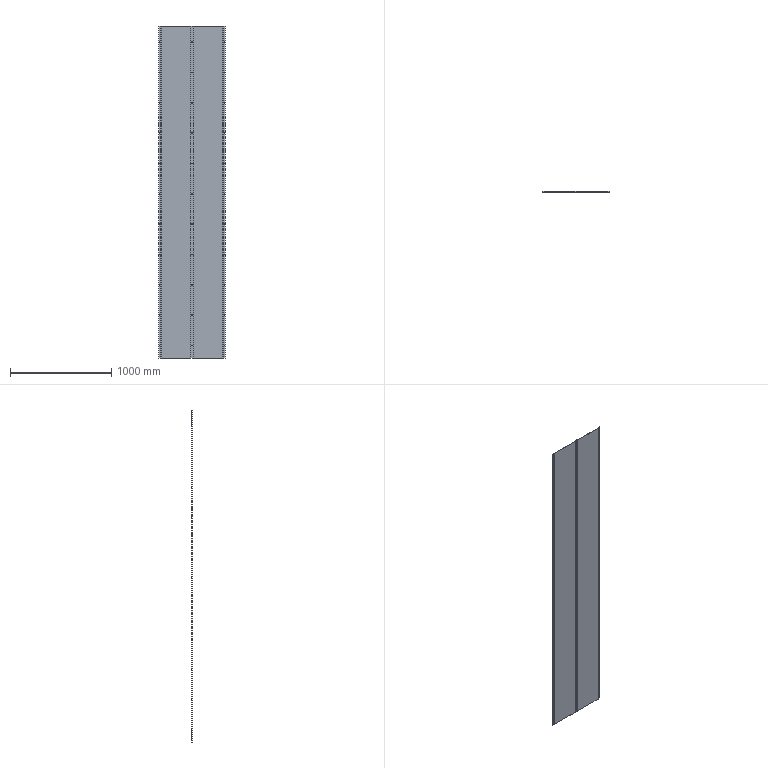Part | STEP file | SX-S16 | 1 solid | 140 faces | box 658 x 4.2 x 3283 mm | volume 2609753 mm3 | cylinder 84 | plane 56 | commonest cylinder face diameters 5.4 x66 0.4 x8 2.8 x8 10 x2